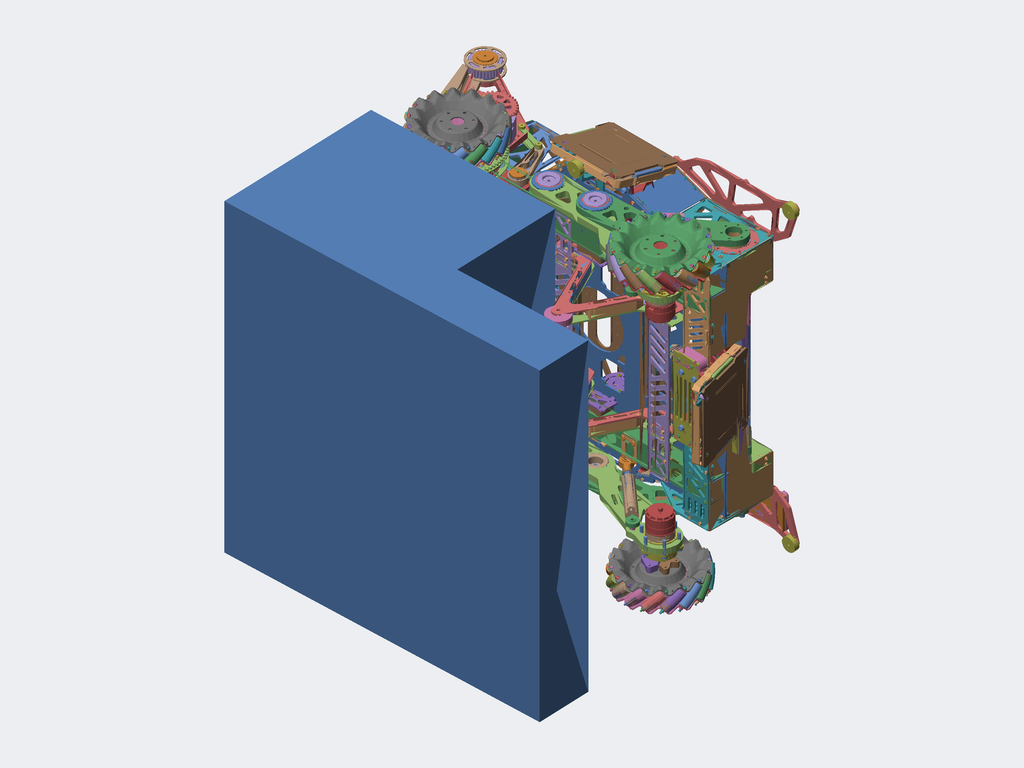Assembly | SolidWorks | 126 different items | 340 placed
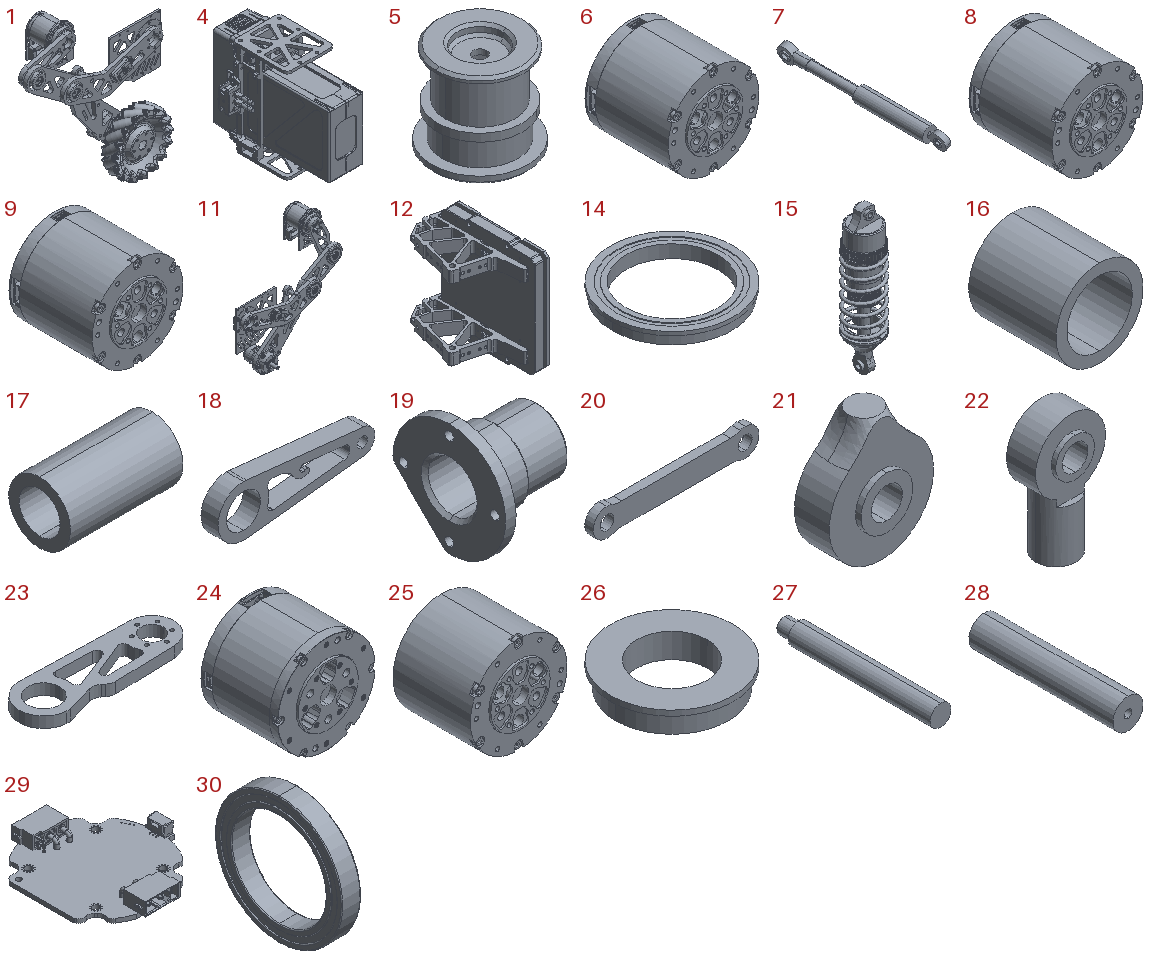Parts list (item | name | quantity | parent item | size | volume | features):
1 | (subassembly) | x1 | - | - | 882461 mm3 | -
2 | (subassembly) | x1 | - | - | - | features CompositeCurve 12, AEMSimFeature 1, CenterOfMass 1
3 | (subassembly) | x1 | in 2 | - | - | -
4 | (subassembly) | x1 | in 2 | - | 356333 mm3 | -
5 | (subassembly) | x4 | in 1, 11 | 37.15 x 37.15 x 35 mm | 13478 mm3 | -
6 | (subassembly) | x2 | in 9 | 57 x 53.3 x 57 mm | 118253 mm3 | -
7 | (subassembly) | x2 | in 1, 11 | - | 32855 mm3 | features CompositeCurve 1
8 | (subassembly) | x2 | in 1, 11 | 57 x 53.3 x 57 mm | 118253 mm3 | -
9 | (subassembly) | x2 | in 8 | 57 x 53.3 x 57 mm | 118253 mm3 | -
10 | (subassembly) | x1 | - | - | - | features CompositeCurve 8
11 | (subassembly) | x1 | - | - | 699438 mm3 | features CompositeCurve 1
12 | (subassembly) | x4 | in 2 | 74.786 x 139.379 x 141 mm | 156127 mm3 | -
13 | (subassembly) | x1 | - | - | - | features CompositeCurve 3
14 | - | x4 | in 10, 13 | 67 x 67 x 7 mm | 9465 mm3 | features ICE 1, Revolution 1
15 | - | x4 | in 10, 13 | 22.605 x 22.6 x 94.05 mm | 15306 mm3 | features BaseBody 4
16 | - | x1 | in 11 | 8 x 8 x 8 mm | 175.929 mm3 | features Extrusion 1
17 | - | x2 | in 1, 11 | 22 x 12 x 12 mm | 1382 mm3 | features Revolution 1
18 | - | x2 | in 10, 13 | 92.5 x 10 x 30 mm | 11719 mm3 | features Fillet 3, ICE 2, Extrusion 1
19 | - | x2 | in 10, 13 | 25 x 31.997 x 31.997 mm | 4923 mm3 | features Chamfer 2, HoleWzd 2, ICE 2, 3DProfileFeature 1, Fillet 1, Revolution 1
20 | - | x4 | in 10, 13 | 60 x 3 x 10 mm | 1346 mm3 | features Extrusion 1, Fillet 1
21 | - | x2 | in 7 | - | 2238 mm3 | features ICE 3, Extrusion 1, Fillet 1
22 | - | x2 | in 7 | 21.7 x 12.5 x 38.85 mm | 4732 mm3 | features ICE 4, Extrusion 1, HoleWzd 1
23 | - | x2 | in 1, 11 | 141.575 x 45.127 x 10 mm | 33796 mm3 | features ICE 3, Fillet 2, Extrusion 1
24 | - | x2 | in 10, 13 | 57 x 46 x 57 mm | 102676 mm3 | features BaseBody 10
25 | - | x2 | in 6 | 57 x 46.8 x 57 mm | 109300 mm3 | features BaseBody 1
26 | - | x4 | in 10, 13 | 35 x 35 x 7 mm | 3667 mm3 | features Extrusion 1, ICE 1
27 | - | x2 | in 7 | 11 x 83 x 11 mm | 7524 mm3 | features Extrusion 1, ICE 1, StudWizard 1
28 | - | x2 | in 7 | 19 x 91 x 19 mm | 18359 mm3 | features Extrusion 1, HoleWzd 1, ICE 1
29 | - | x2 | in 6 | - | - | features RefSurface 1
30 | - | x2 | in 1, 11 | 7 x 47 x 47 mm | 4099 mm3 | features Revolution 5, CirPattern 2, RefAxis 1, RevCut 1
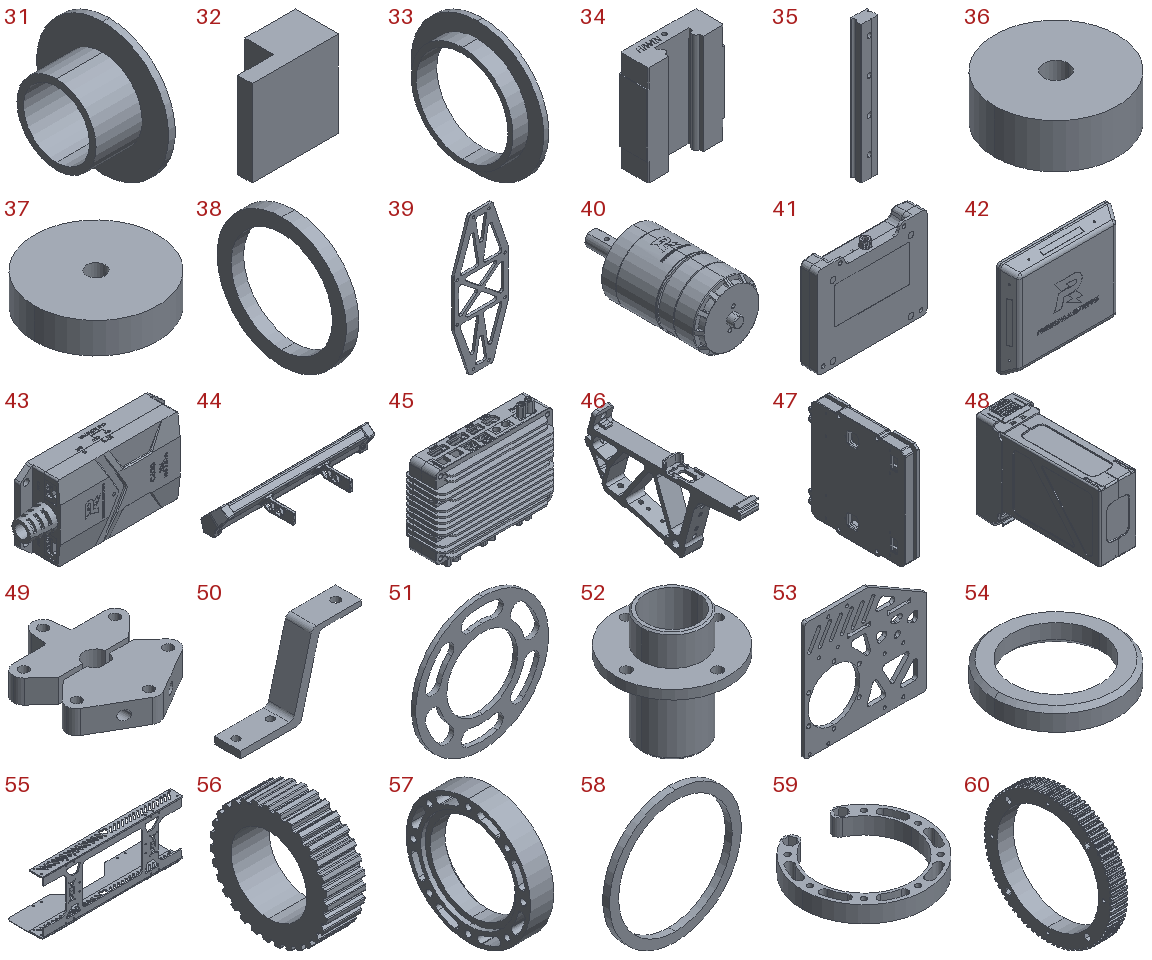31 | - | x8 | in 10, 13 | 4 x 10 x 10 mm | 59.69 mm3 | features Revolution 1
32 | - | x1 | - | 600 x 300 x 600 mm | 78000000 mm3 | features Extrusion 1
33 | - | x4 | in 10, 13 | 4 x 26 x 26 mm | 455.531 mm3 | features Revolution 1
34 | - | x8 | in 10, 13 | 27 x 10 x 34.7 mm | 7013 mm3 | features BaseBody 1
35 | - | x4 | in 10, 13 | 12 x 8 x 100 mm | 8420 mm3 | features ICE 3, BaseBody 1
36 | - | x4 | in 2 | 25 x 25 x 9 mm | 4241 mm3 | features Revolution 1
37 | - | x2 | in 2 | 40 x 40 x 10 mm | 12284 mm3 | features Revolution 1
38 | - | x2 | in 1, 11 | 5 x 51 x 51 mm | 3931 mm3 | features Revolution 1
39 | - | x1 | in 2 | 70 x 3 x 180 mm | 15170 mm3 | features ICE 2, Extrusion 1, Fillet 1
40 | - | x4 | in 1, 10, 11, 13 | 42 x 98.4 x 44.727 mm | 85611 mm3 | features BaseBody 17
41 | - | x1 | in 2 | 76 x 15.355 x 63 mm | 45153 mm3 | features BaseBody 13, DeleteBody 1, Revolution 1
42 | - | x1 | in 2 | 121.675 x 17.8 x 105.675 mm | 74088 mm3 | features BaseBody 6
43 | - | x4 | in 1, 2, 11 | 53.7 x 11.5 x 26.125 mm | 11767 mm3 | features BaseBody 25, DeleteBody 2, RefSurface 1
44 | - | x1 | in 2 | 285 x 84.728 x 49.99 mm | 138655 mm3 | features BaseBody 32, SewRefSurface 2, Thicken 2, DeleteBody 1, ICE 1
45 | - | x1 | in 2 | - | - | features BaseBody 45, RefSurface 2, DeleteBody 1
46 | - | x8 | in 12 | 15 x 130.973 x 68.389 mm | 25082 mm3 | features BaseBody 1
47 | - | x4 | in 12 | 19 x 129.965 x 141 mm | 105960 mm3 | features BaseBody 16, Blend 1, Shell 1
48 | - | x1 | in 4 | 44.3 x 134.8 x 101.5 mm | 316528 mm3 | features BaseBody 10
49 | - | x4 | in 1, 10, 11, 13 | 47.971 x 54.2 x 10 mm | 13527 mm3 | features BaseBody 2
50 | - | x2 | in 2 | 70.55 x 15 x 45 mm | 6219 mm3 | features Extrusion 1, Fillet 1, ICE 1
51 | - | x4 | in 10, 13 | 60 x 2 x 60 mm | 2573 mm3 | features Extrusion 1, ICE 1
52 | - | x2 | in 10, 13 | 37 x 37 x 36.5 mm | 6267 mm3 | features ICE 4, Chamfer 2, HoleWzd 2, 3DProfileFeature 1, Extrusion 1
53 | - | x2 | in 1, 11 | 130 x 4 x 126 mm | 41493 mm3 | features ICE 5, Fillet 2, Extrusion 1
54 | - | x8 | in 5 | 38 x 38 x 6.3 mm | 3255 mm3 | features Chamfer 2, Extrusion 1
55 | - | x1 | in 2 | 363 x 91.15 x 140 mm | 130923 mm3 | features ICE 5, Fillet 2, Extrusion 1, MirrorSolid 1
56 | - | x2 | in 10, 13 | 16 x 49.566 x 49.615 mm | 16375 mm3 | features CirPattern 1, Cut 1, ICE 1, RefAxis 1, Revolution 1
57 | - | x1 | in 10 | 16 x 85 x 85 mm | 32635 mm3 | features ICE 1, Revolution 1
58 | - | x2 | in 10, 13 | 58 x 3 x 58 mm | 2036 mm3 | features Extrusion 1
59 | - | x1 | in 10 | 74 x 70.267 x 10 mm | 10018 mm3 | features ICE 2, Extrusion 1, Fillet 1
60 | - | x2 | in 10, 13 | 16 x 125.578 x 125.622 mm | 66600 mm3 | features ICE 3, Cut 2, Chamfer 1, CirPattern 1, RefAxis 1, Revolution 1
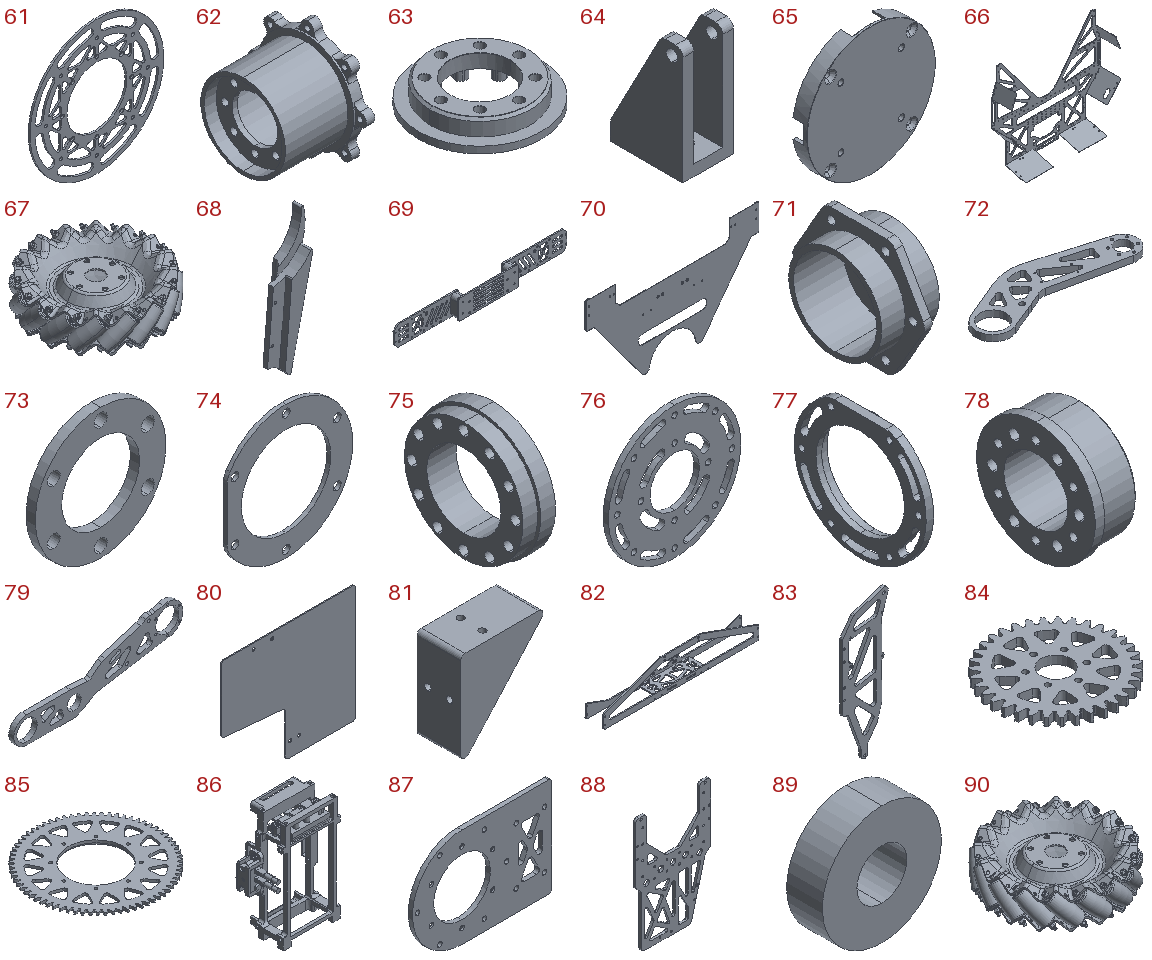61 | - | x4 | in 10, 13 | 145 x 2 x 145 mm | 15235 mm3 | features CirPattern 1, Extrusion 1, Fillet 1, ICE 1
62 | - | x2 | in 10, 13 | 43 x 70 x 70 mm | 21080 mm3 | features ICE 4, HoleWzd 1, Revolution 1
63 | - | x1 | in 10 | 55 x 55 x 10.2 mm | 10014 mm3 | features ICE 3, Chamfer 1, Fillet 1, Revolution 1
64 | - | x4 | in 10, 13 | 14 x 20 x 32 mm | 3086 mm3 | features ICE 4, Extrusion 1, Fillet 1
65 | - | x2 | in 6 | 57 x 6.5 x 57 mm | 5262 mm3 | features BaseBody 1
66 | - | x1 | in 2 | 486 x 96.259 x 428.466 mm | 244289 mm3 | features ICE 8, Fillet 4, Extrusion 1, MirrorSolid 1
67 | - | x2 | in 11, 13 | 152.394 x 152.394 x 45.547 mm | 219061 mm3 | features BaseBody 146
68 | - | x2 | in 10, 13 | 70.208 x 32 x 213.495 mm | 127310 mm3 | features ICE 3, Fillet 2, DelFace 1, Extrusion 1, MirrorSolid 1
69 | - | x1 | in 2 | 433.1 x 23 x 50 mm | 82463 mm3 | features ICE 8, Fillet 7, Chamfer 1, Extrusion 1
70 | - | x1 | in 2 | 441.1 x 3 x 236.71 mm | 53782 mm3 | features ICE 2, Extrusion 1, Fillet 1, MirrorSolid 1
71 | - | x2 | in 1, 11 | 29.45 x 67.158 x 59.5 mm | 18545 mm3 | features ICE 3, Fillet 1, Revolution 1
72 | - | x2 | in 1, 11 | 255.5 x 84.429 x 10 mm | 83626 mm3 | features ICE 7, Fillet 2, Extrusion 1
73 | - | x2 | in 1, 11 | 42 x 3 x 42 mm | 2434 mm3 | features Extrusion 1
74 | - | x2 | in 1, 11 | 66 x 2 x 70 mm | 3883 mm3 | features Extrusion 1
75 | - | x2 | in 1, 11 | 9.95 x 42 x 42 mm | 7242 mm3 | features HoleWzd 1, Revolution 1
76 | - | x2 | in 10, 13 | 75 x 3 x 75 mm | 8695 mm3 | features Extrusion 1, ICE 1
77 | - | x2 | in 1, 11 | 8 x 70 x 66 mm | 7364 mm3 | features ICE 2, Chamfer 1, Fillet 1, HoleWzd 1, Revolution 1
78 | - | x2 | in 1, 11 | 14 x 37 x 37 mm | 7882 mm3 | features ICE 2, Chamfer 1, HoleWzd 1, Revolution 1
79 | - | x2 | in 1, 11 | 347.966 x 10 x 110.45 mm | 118705 mm3 | features ICE 5, Fillet 2, Extrusion 1
80 | - | x2 | in 2 | 144.55 x 1 x 127 mm | 14747 mm3 | features Extrusion 1, Fillet 1
81 | - | x2 | in 2 | 37.777 x 20 x 41.764 mm | 17216 mm3 | features ICE 2, Extrusion 1, Fillet 1
82 | - | x1 | in 2 | 433.1 x 53 x 95 mm | 77453 mm3 | features Fillet 6, ICE 4, Extrusion 1
83 | - | x2 | in 2 | 81.5 x 5 x 248 mm | 38824 mm3 | features Fillet 3, ICE 3, Chamfer 1, Extrusion 1
84 | - | x2 | in 10, 13 | 73.978 x 73.911 x 5 mm | 13896 mm3 | features ICE 3, CirPattern 1, Extrusion 1, RefAxis 1
85 | - | x2 | in 10, 13 | 144 x 143.917 x 5 mm | 31123 mm3 | features ICE 4, CirPattern 1, Extrusion 1, HoleWzd 1, RefAxis 1
86 | - | x1 | in 4 | 69.4 x 39.5 x 103.5 mm | 27545 mm3 | features BaseBody 12
87 | - | x2 | in 1, 11 | 98.2 x 3 x 70 mm | 13699 mm3 | features ICE 2, 3DProfileFeature 1, Extrusion 1, Fillet 1, HoleWzd 1
88 | - | x2 | in 10, 13 | 133 x 4 x 208.15 mm | 51561 mm3 | features ICE 8, Fillet 4, Chamfer 1, Extrusion 1
89 | - | x2 | in 2 | 10 x 3 x 10 mm | 194.056 mm3 | features Extrusion 1
90 | - | x2 | in 1, 10 | 152.18 x 152.18 x 45.547 mm | 218308 mm3 | features BaseBody 114, ICE 1
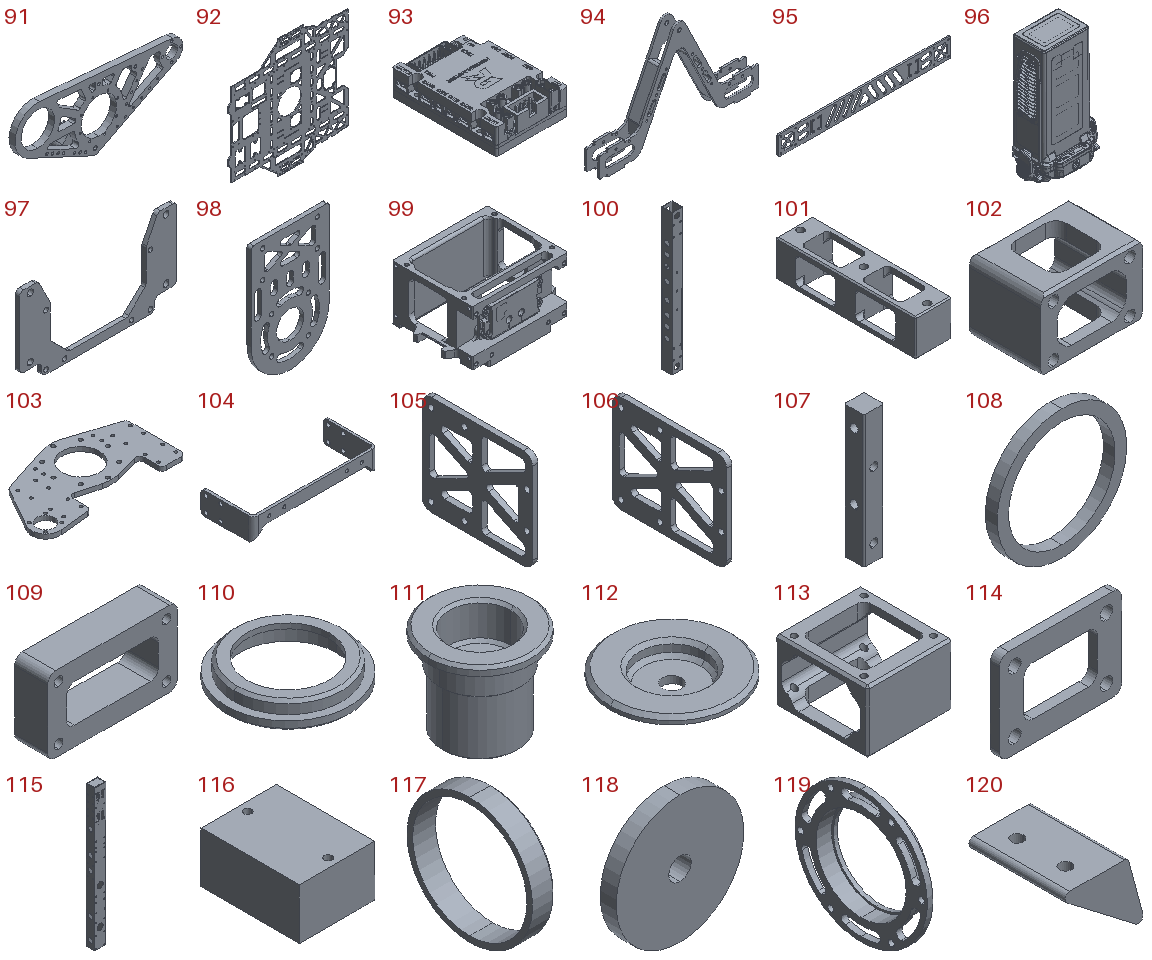91 | - | x2 | in 10, 13 | 276 x 41 x 121.736 mm | 133233 mm3 | features ICE 8, Fillet 5, Extrusion 1, MirrorSolid 1
92 | - | x1 | in 2 | 510.5 x 3 x 508 mm | 398593 mm3 | features ICE 16, Fillet 6, Chamfer 2, Extrusion 1
93 | - | x1 | in 2 | - | 22685 mm3 | features BaseBody 8
94 | - | x2 | in 2 | 239 x 22 x 147.217 mm | 68653 mm3 | features ICE 5, Extrusion 1, Fillet 1, MirrorSolid 1
95 | - | x2 | in 2 | 355 x 3 x 40 mm | 28604 mm3 | features ICE 3, Extrusion 1, Fillet 1
96 | - | x1 | in 3 | - | - | features RefSurface 17, Attribute 3
97 | - | x1 | in 2 | 110 x 3 x 59 mm | 7718 mm3 | features Chamfer 2, Extrusion 1, Fillet 1
98 | - | x2 | in 1, 11 | 57 x 3 x 91.7 mm | 10337 mm3 | features Extrusion 1, Fillet 1, ICE 1
99 | - | x1 | in 3 | - | - | features BaseBody 126, RefSurface 28, Attribute 3
100 | - | x2 | in 2 | 30 x 30 x 415 mm | 44267 mm3 | features ICE 3, Extrusion 1, Shell 1
101 | - | x2 | in 2 | 28 x 106 x 28 mm | 37370 mm3 | features ICE 2, Chamfer 1, Extrusion 1
102 | - | x4 | in 2 | 40 x 28 x 28 mm | 13306 mm3 | features ICE 3, Fillet 2, Chamfer 1, Extrusion 1
103 | - | x2 | in 10, 13 | 163.5 x 91 x 5 mm | 40085 mm3 | features ICE 10, Fillet 5, MirrorPattern 2, Extrusion 1
104 | - | x1 | in 2 | 100 x 41.788 x 18 mm | 4551 mm3 | features Fillet 1, FlatPattern 1, HoleWzd 1, SM3dBend 1, SMBaseFlange 1, SheetMetal 1
105 | - | x1 | in 4 | 3 x 61 x 55 mm | 5958 mm3 | features Fillet 2, ICE 2, Extrusion 1
106 | - | x1 | in 4 | 3 x 64.5 x 55 mm | 6303 mm3 | features Fillet 2, ICE 2, Extrusion 1
107 | - | x50 | in 2, 10 | 6 x 6 x 40 mm | 1314 mm3 | features HoleWzd 2, Extrusion 1, Fillet 1
108 | - | x4 | in 5 | 33 x 3 x 33 mm | 829.092 mm3 | features Extrusion 1
109 | - | x2 | in 1, 11 | 48 x 12.25 x 28 mm | 10214 mm3 | features Extrusion 1
110 | - | x8 | in 5 | 48 x 48 x 8.3 mm | 4148 mm3 | features Chamfer 2, ICE 2, Extrusion 1
111 | - | x4 | in 5 | 37.15 x 37.15 x 32.5 mm | 10461 mm3 | features Chamfer 5, ICE 4, 3DProfileFeature 1, Extrusion 1, HoleWzd 1
112 | - | x4 | in 5 | 34 x 34 x 6 mm | 2188 mm3 | features Chamfer 2, ICE 2, Extrusion 1
113 | - | x4 | in 2 | 37 x 40 x 27 mm | 11447 mm3 | features ICE 3, 3DProfileFeature 1, Chamfer 1, Extrusion 1, HoleWzd 1
114 | - | x4 | in 2 | 40 x 3 x 30 mm | 2282 mm3 | features Extrusion 1
115 | - | x2 | in 2 | 40 x 30 x 505 mm | 171270 mm3 | features ICE 9, Chamfer 1, Extrusion 1, Fillet 1
116 | - | x2 | in 2 | 44.5 x 58 x 30 mm | 76476 mm3 | features Extrusion 1
117 | - | x4 | in 10, 13 | 10 x 55 x 55 mm | 4038 mm3 | features Chamfer 1, Revolution 1
118 | - | x4 | in 10, 13 | 24 x 3 x 24 mm | 1316 mm3 | features Extrusion 1
119 | - | x2 | in 1, 11 | 10 x 69 x 69 mm | 6569 mm3 | features ICE 2, Revolution 1
120 | - | x2 | in 2 | 16.208 x 20 x 12.902 mm | 1998 mm3 | features Extrusion 1, Fillet 1, HoleWzd 1, MirrorPattern 1
121 | hex nuts, style 1-grades ab gb | x1 | - | - | - | -
122 | hexagon socket button head screws gb | x1 | - | - | - | -
123 | hexagon socket countersunk head screws gb | x1 | - | - | - | -
124 | hexagon socket head cap screws gb | x1 | - | - | - | -
125 | hexagon socket head shoulder screws gb | x1 | - | - | - | -
126 | Shoulder Bolt | x1 | - | - | - | -
Mates (type | each side: item.copy, entity, surface, feature), first 384 of 755 lines:
In the top assembly
Coincident | 115.1 face plane Boss-Extrude 1 | 88.1 face plane Boss-Extrude 1
Concentric | 115.1 face cylinder Cut-Extrude 2 | 88.1 face cylinder Cut-Extrude 3
Concentric | 115.1 face cylinder Cut-Extrude 2 | 15.1 face cylinder Shock Absorber-85mm Thickened Center Shaft-1-solid1
Coincident | 115.2 face plane Boss-Extrude 1 | 88.2 face plane Boss-Extrude 1
Concentric | 115.2 face cylinder Cut-Extrude 2 | 15.2 face cylinder Shock Absorber-85mm Thickened Center Shaft-1-solid1
Concentric | 115.2 face cylinder Cut-Extrude 2 | 15.3 face cylinder Shock Absorber-85mm Thickened Center Shaft-1-solid1
Coincident | 115.1 face plane Boss-Extrude 1 | 87.1 face plane Boss-Extrude 1
Concentric | 115.1 face cylinder Cut-Extrude 4 | 87.1 face cylinder Boss-Extrude 1 | 2 times
Concentric | 107.1 face cylinder M3 Tapped Hole 2 | 53.1 face cylinder Boss-Extrude 1
Coincident | 115.2 face plane Boss-Extrude 1 | 87.2 face plane Boss-Extrude 1
Concentric | 115.2 face cylinder Cut-Extrude 4 | 87.2 face cylinder Boss-Extrude 1 | 2 times
Concentric | 107.2 face cylinder M3 Tapped Hole 2 | 53.2 face cylinder Boss-Extrude 1 | 2 times
Concentric | 107.3 face cylinder M3 Tapped Hole 1 | 53.1 face cylinder Cut-Extrude 1 | 2 times
Concentric | 107.4 face cylinder M3 Tapped Hole 2 | 53.2 face cylinder Cut-Extrude 1
Concentric | 72.1 face cylinder Boss-Extrude 1 | 72.2 face cylinder Boss-Extrude 1
Concentric | 91.1 face cylinder Boss-Extrude 1 | 91.2 face cylinder Boss-Extrude 1
Coincident | 100.1 face plane Boss-Extrude 1 | assembly face
Coincident | 2.1 plane | 32.1 plane
Tangent | 37.1 face cylinder Revolve 1 | 32.1 face plane Boss-Extrude 1
Tangent | 90.1 select_type:24 | 32.1 face plane Boss-Extrude 1
Parallel | 92.1 select_type:24 | 32.1 face plane Boss-Extrude 1
Concentric | 115.2 face cylinder Cut-Extrude 3 | assembly face
Coincident | 115.2 face plane Boss-Extrude 1 | assembly face
Coincident | 53.2 face plane Boss-Extrude 1 | assembly face | 2 times
Concentric | 53.2 face cylinder Boss-Extrude 1 | assembly face
Coincident | 88.2 face plane Boss-Extrude 1 | assembly face
Concentric | 100.1 face cylinder Cut-Extrude 1 | assembly face | 2 times
In subassembly 2
Coincident | 92.2 face plane Boss-Extrude 1 | 115.3 face plane Boss-Extrude 1
Coincident | 92.2 face plane Boss-Extrude 1 | 115.4 face plane Boss-Extrude 1
Coincident | 115.3 face plane Boss-Extrude 1 | 2.2 face | 3 times
Concentric | 115.3 face cylinder Cut-Extrude 2 | 2.2 face | 4 times
Concentric | 2.2 face | 2.2 face | 10 times
Coincident | 115.4 face plane Boss-Extrude 1 | 2.2 face | 2 times
Concentric | 115.4 face cylinder Cut-Extrude 2 | 2.2 face | 3 times
Concentric | 2.2 face | 107.5 face cylinder M3 Tapped Hole 2 | 2 times
Coincident | 2.2 face | 107.5 face plane Boss-Extrude 1
Coincident | 2.2 face | 2.2 face | 9 times
Concentric | 92.2 face cylinder Cut-Extrude 1 | 46.1 face cylinder Import 1
Concentric | 92.2 face cylinder Cut-Extrude 1 | 46.2 face cylinder Import 1
Coincident | 2.2 edge | 2.2 edge
Concentric | 92.2 face cylinder Cut-Extrude 2 | 115.3 face cylinder Cut-Extrude 3 | 2 times
Coincident | 92.2 face plane Boss-Extrude 1 | 46.1 face plane Import 1
Concentric | 2.2 face | 55.1 face cylinder Mirror 1 | 2 times
Concentric | 92.2 face cylinder Cut-Extrude 2 | 115.4 face cylinder Cut-Extrude 3 | 2 times
Concentric | 55.1 face cylinder Boss-Extrude 2 | 2.2 face | 3 times
Concentric | 55.1 face cylinder Boss-Extrude 2 | 107.6 face cylinder M3 Tapped Hole 1 | 2 times
Concentric | 2.2 face | 107.6 face cylinder M3 Tapped Hole 2
Coincident | 2.2 face | 55.1 face plane Mirror 1
Coincident | 92.2 face plane Boss-Extrude 1 | 2.2 face | 6 times
Coincident | 46.2 face plane Import 1 | 46.3 face plane Import 1
Tangent | 2.2 select_type:0 | 2.2 face
Concentric | 115.3 face cylinder Cut-Extrude 4 | 2.2 face | 2 times
Coincident | 92.2 face plane Boss-Extrude 1 | 46.4 face plane Import 1
Concentric | 92.2 face cylinder Boss-Extrude 2 | 46.4 face cylinder Import 1
Concentric | 92.2 face cylinder Boss-Extrude 2 | 46.5 face cylinder Import 1
Coincident | 92.2 select_type:24 | 2.2 face | 2 times
Coincident | 2.2 plane | 2.2 plane
Concentric | 46.3 face cylinder Import 1 | 2.2 face | 2 times
Coincident | 92.2 face plane Boss-Extrude 1 | 100.2 face plane Boss-Extrude 1
Coincident | 92.2 face plane Boss-Extrude 1 | 100.3 face plane Boss-Extrude 1
Coincident | 92.2 face plane Boss-Extrude 2 | 100.3 face plane Boss-Extrude 1
Parallel | 46.6 face plane Import 1 | 44.1 face plane Import 22 | 2 times
Concentric | 46.3 face cylinder Import 1 | 69.1 face cylinder Boss-Extrude 3
Concentric | 46.6 face cylinder Import 1 | 69.1 face cylinder Boss-Extrude 3
Coincident | 46.6 face plane Import 1 | 69.1 face plane Boss-Extrude 3
Coincident | 115.3 face plane Boss-Extrude 1 | 69.1 face plane Boss-Extrude 1
Coincident | 55.1 face plane Boss-Extrude 2 | 2.2 face
Coincident | 55.1 face plane Boss-Extrude 2 | 107.6 face plane Boss-Extrude 1
Concentric | 107.5 face cylinder M3 Tapped Hole 1 | 55.1 face cylinder Mirror 1 | 2 times
Coincident | 107.5 face plane Boss-Extrude 1 | 55.1 face plane Mirror 1
Concentric | 69.1 face cylinder Cut-Extrude 1 | 107.7 edge
Concentric | 2.2 face | 107.7 face cylinder M3 Tapped Hole 2
Concentric | 92.2 face cylinder Cut-Extrude 4 | 107.8 face cylinder M3 Tapped Hole 1 | 2 times
Concentric | 2.2 face | 107.8 face cylinder M3 Tapped Hole 2
Concentric | 46.6 face cylinder Import 1 | 82.1 face cylinder Boss-Extrude 1 | 2 times
Coincident | 46.6 face plane Import 1 | 82.1 face plane Boss-Extrude 1
Coincident | 82.1 face plane Boss-Extrude 1 | 2.2 face
Parallel | 46.1 face plane Import 1 | 86.1 face plane DJI Battery Holder 2017-1-solid1
Coincident | 82.1 face plane Boss-Extrude 1 | 107.9 face plane Boss-Extrude 1
Concentric | 82.1 face cylinder Cut-Extrude 1 | 107.9 edge
Concentric | 82.1 face cylinder Boss-Extrude 2 | 107.9 face cylinder M3 Tapped Hole 2
Coincident | 82.1 face plane Boss-Extrude 3 | 104.1 face plane Base-Flange 1
Coincident | 44.1 face plane Import 22 | 82.1 face plane Boss-Extrude 2
Concentric | 82.1 face cylinder Boss-Extrude 3 | 104.1 face cylinder M3 Tapped Hole 2 | 2 times
Coincident | 44.1 face plane Import 22 | 104.1 face plane Sketched Bend 2
Concentric | 44.1 face cylinder Cut-Extrude 1 | 104.1 face cylinder Base-Flange 1 | 2 times
Coincident | 82.1 face plane Boss-Extrude 1 | 107.10 face plane Boss-Extrude 1
Concentric | 82.1 face cylinder Boss-Extrude 2 | 107.10 face cylinder M3 Tapped Hole 1
Concentric | 82.1 face cylinder Cut-Extrude 1 | 107.10 face cylinder M3 Tapped Hole 2
Coincident | 82.1 face plane Boss-Extrude 2 | 107.11 face plane Boss-Extrude 1
Concentric | 82.1 face cylinder Boss-Extrude 3 | 107.11 face cylinder M3 Tapped Hole 2
Concentric | 82.1 face cylinder Boss-Extrude 2 | 107.11 face cylinder M3 Tapped Hole 1
Concentric | 82.1 face cylinder Boss-Extrude 2 | 107.12 face cylinder M3 Tapped Hole 2
Concentric | 82.1 face cylinder Boss-Extrude 3 | 107.12 face cylinder M3 Tapped Hole 1
Coincident | 92.2 face plane Boss-Extrude 1 | 107.8 face plane Boss-Extrude 1
Concentric | 82.1 face cylinder Boss-Extrude 3 | 107.13 face cylinder M3 Tapped Hole 2 | 2 times
Coincident | 82.1 face plane Boss-Extrude 3 | 107.13 face plane Boss-Extrude 1
Coincident | 82.1 face plane Boss-Extrude 1 | 107.14 face plane Boss-Extrude 1
Concentric | 82.1 face cylinder Cut-Extrude 1 | 107.14 face cylinder M3 Tapped Hole 2 | 2 times
Concentric | 46.4 face cylinder Import 1 | 66.1 face cylinder Boss-Extrude 1
Concentric | 46.2 face cylinder Import 1 | 66.1 face cylinder Boss-Extrude 1
Coincident | 46.5 face plane Import 1 | 66.1 face plane Boss-Extrude 1
Coincident | 2.2 face | 107.15 face plane Boss-Extrude 1
Concentric | 46.1 face cylinder Import 1 | 97.1 face cylinder Boss-Extrude 1 | 2 times
Coincident | 46.2 face plane Import 1 | 97.1 face plane Boss-Extrude 1
Coincident | 92.2 face plane Boss-Extrude 1 | 46.7 face plane Import 1
Concentric | 92.2 face cylinder Boss-Extrude 2 | 46.7 face cylinder Import 1 | 2 times
Coincident | 92.2 select_type:25 | 2.2 axis | 2 times
Coincident | 100.3 face plane Boss-Extrude 1 | 2.2 face | 4 times
Concentric | 100.3 face cylinder Cut-Extrude 1 | 2.2 face | 3 times
Concentric | 100.3 edge | 2.2 face
Concentric | 100.2 face cylinder Cut-Extrude 1 | 2.2 face | 2 times
Concentric | 92.2 face cylinder Cut-Extrude 6 | 100.2 face cylinder Cut-Extrude 1 | 2 times
Concentric | 92.2 face cylinder Cut-Extrude 6 | 100.3 face cylinder Cut-Extrude 1
Coincident | 66.1 face plane Boss-Extrude 3 | 107.16 face plane Boss-Extrude 1
Concentric | 66.1 face cylinder Boss-Extrude 3 | 107.16 face cylinder M3 Tapped Hole 2 | 2 times
Concentric | 2.2 face | 107.15 face cylinder M3 Tapped Hole 1 | 2 times
Concentric | 107.15 face cylinder M3 Tapped Hole 2 | 70.1 face cylinder Boss-Extrude 1 | 2 times
Coincident | 107.15 face plane Boss-Extrude 1 | 70.1 face plane Boss-Extrude 1
Coincident | 69.1 face plane Boss-Extrude 1 | 80.1 face plane Boss-Extrude 1
Coincident | 66.1 face plane Boss-Extrude 5 | 120.1 face plane Boss-Extrude 1
Concentric | 66.1 face cylinder Cut-Extrude 2 | 120.1 face cylinder Mirror 1 | 2 times
Coincident | 99.1 face plane battery_rack.stp-1/_V06-202409130001_ASM_12_ASM.stp-1/DCJ-V13-20241024_13.stp-1-solid1 | 97.1 face plane Boss-Extrude 1
Concentric | 99.1 face cylinder battery_rack.stp-1/_V06-202409130001_ASM_12_ASM.stp-1/DCJ-V13-20241024_13.stp-1-solid1 | 97.1 face cylinder Boss-Extrude 1 | 2 times
Coincident | 80.1 face plane Boss-Extrude 1 | 81.1 face plane Boss-Extrude 1
Coincident | 70.1 face plane Boss-Extrude 1 | 81.1 face plane Boss-Extrude 1 | 2 times
Concentric | 80.1 face cylinder Boss-Extrude 1 | 81.1 face cylinder Cut-Extrude 2 | 2 times
Concentric | 69.1 face cylinder Boss-Extrude 1 | 107.17 face cylinder M3 Tapped Hole 1
Concentric | 80.1 face cylinder Boss-Extrude 1 | 107.17 face cylinder M3 Tapped Hole 2
Concentric | 69.1 face cylinder Boss-Extrude 1 | 107.18 face cylinder M3 Tapped Hole 2 | 2 times
Coincident | 69.1 face plane Boss-Extrude 1 | 107.18 face plane Boss-Extrude 1
Concentric | 80.2 face cylinder Boss-Extrude 1 | 107.18 face cylinder M3 Tapped Hole 1 | 2 times
Coincident | 80.2 face plane Boss-Extrude 1 | 107.18 face plane Boss-Extrude 1
Coincident | 80.2 face plane Boss-Extrude 1 | 81.2 face plane Boss-Extrude 1
Concentric | 80.2 face cylinder Boss-Extrude 1 | 81.2 face cylinder Cut-Extrude 2 | 2 times
Coincident | 66.1 face plane Boss-Extrude 1 | 83.1 face plane Boss-Extrude 1
Concentric | 70.1 face cylinder Boss-Extrude 1 | 83.1 face cylinder Boss-Extrude 1
Concentric | 46.5 face cylinder Import 1 | 83.1 face cylinder Boss-Extrude 1
Coincident | 83.1 face plane Boss-Extrude 1 | 41.1 face plane Import 5
Concentric | 83.1 face cylinder Boss-Extrude 2 | 41.1 face cylinder Import 5
Concentric | 83.1 face cylinder Cut-Extrude 3 | 41.1 face cylinder Import 5
Concentric | 46.8 face cylinder Import 1 | 83.2 face cylinder Boss-Extrude 1
Concentric | 70.1 face cylinder Boss-Extrude 1 | 83.2 face cylinder Boss-Extrude 1
Coincident | 66.1 face plane Boss-Extrude 1 | 83.2 face plane Boss-Extrude 1
Coincident | 83.1 face plane Boss-Extrude 1 | 36.1 face plane Revolve 1
Concentric | 83.1 face cylinder Boss-Extrude 1 | 36.1 edge
Coincident | 92.2 face plane Boss-Extrude 1 | 50.1 face plane Boss-Extrude 1
Concentric | 92.2 face cylinder Boss-Extrude 2 | 50.1 face cylinder Cut-Extrude 1 | 2 times
Concentric | 50.1 face cylinder Cut-Extrude 1 | 36.2 face cylinder Revolve 1
Coincident | 92.2 face plane Boss-Extrude 1 | 50.2 face plane Boss-Extrude 1
Concentric | 92.2 face cylinder Boss-Extrude 2 | 50.2 face cylinder Cut-Extrude 1 | 2 times
Coincident | 50.2 face plane Boss-Extrude 1 | 36.3 face plane Revolve 1
Concentric | 50.2 face cylinder Cut-Extrude 1 | 36.3 face cylinder Revolve 1
Coincident | 92.2 face plane Boss-Extrude 1 | 94.1 face plane Boss-Extrude 1
Coincident | 92.2 face plane Support Guide Wheel Mount | 94.1 face plane Boss-Extrude 1 | 2 times
Tangent | 2.2 face | 94.1 select_type:24
Concentric | 115.3 face cylinder Cut-Extrude 3 | 95.1 face cylinder Boss-Extrude 1 | 2 times
Coincident | 115.3 face plane Boss-Extrude 1 | 95.2 face plane Boss-Extrude 1
Concentric | 115.3 face cylinder Cut-Extrude 3 | 95.2 face cylinder Boss-Extrude 1 | 2 times
Concentric | 94.1 face cylinder Boss-Extrude 1 | 2.2 face
Concentric | 94.2 face cylinder Boss-Extrude 1 | 2.2 face
Coincident | 95.1 face plane Boss-Extrude 1 | 2.2 face | 4 times
Coincident | 95.1 face plane Boss-Extrude 1 | 94.2 face plane Boss-Extrude 1 | 2 times
Concentric | 42.1 face cylinder Import 2 | 39.1 face cylinder Cut-Extrude 1 | 2 times
Coincident | 42.1 face plane Import 2 | 39.1 face plane Boss-Extrude 1
Concentric | 55.1 face cylinder Cut-Extrude 1 | 39.1 face cylinder Cut-Extrude 1 | 2 times
Coincident | 55.1 face plane Boss-Extrude 1 | 39.1 face plane Boss-Extrude 1
Concentric | 83.2 face cylinder Boss-Extrude 1 | 36.4 face cylinder Revolve 1
Coincident | 83.2 face plane Boss-Extrude 1 | 36.4 face plane Revolve 1
Width | 94.1 face plane Boss-Extrude 1 | 2.2 face | 37.2 face plane Revolve 1 | 37.2 face plane Revolve 1
Concentric | 2.2 face | 37.2 face cylinder Revolve 1
Concentric | 94.2 face cylinder Boss-Extrude 1 | 37.3 face cylinder Revolve 1
Width | 2.2 face | 94.2 face plane Boss-Extrude 1 | 37.3 face plane Revolve 1 | 37.3 face plane Revolve 1
Coincident | 50.1 face plane Boss-Extrude 1 | 36.2 face plane Revolve 1
Concentric | 95.1 face cylinder Cut-Extrude 2 | 107.19 face cylinder M3 Tapped Hole 1
Concentric | 94.1 face cylinder Cut-Extrude 3 | 107.19 face cylinder M3 Tapped Hole 2
Coincident | 94.1 face plane Mirror 1 | 95.1 face plane Boss-Extrude 1
Concentric | 94.1 face cylinder Boss-Extrude 1 | 37.2 face cylinder Revolve 1
Coincident | 95.1 face plane Boss-Extrude 1 | 94.2 face plane Mirror 1
Concentric | 100.2 face cylinder Cut-Extrude 1 | 102.1 face cylinder Cut-Extrude 1 | 2 times
Coincident | 100.2 face plane Shell 1 | 102.1 face plane Boss-Extrude 1
Coincident | 100.3 face plane Shell 1 | 102.2 face plane Boss-Extrude 1
Concentric | 100.3 face cylinder Cut-Extrude 1 | 102.2 face cylinder Cut-Extrude 1 | 2 times
Coincident | 115.3 face plane Boss-Extrude 1 | 113.1 face plane Boss-Extrude 1
Concentric | 115.3 face cylinder Cut-Extrude 3 | 113.1 face cylinder Cut-Extrude 3 | 2 times
Concentric | 100.2 face cylinder Cut-Extrude 1 | 101.1 face cylinder Cut-Extrude 1 | 2 times
Coincident | 100.2 face plane Shell 1 | 101.1 face plane Boss-Extrude 1
Concentric | 115.3 face cylinder Cut-Extrude 5 | 114.1 face cylinder Boss-Extrude 1 | 2 times
Coincident | 115.3 face plane Boss-Extrude 1 | 114.1 face plane Boss-Extrude 1
Concentric | 92.2 face cylinder Conduit Mount | 45.1 face cylinder Import 24 | 2 times
Coincident | 92.2 face plane Boss-Extrude 1 | 45.1 face plane Import 24
Concentric | 69.1 face cylinder Cut-Extrude 1 | 107.7 face cylinder M3 Tapped Hole 1
Coincident | 82.1 face plane Boss-Extrude 3 | 70.1 face plane Boss-Extrude 1
Concentric | 82.1 face cylinder Cut-Extrude 1 | 107.20 face cylinder M3 Tapped Hole 2 | 2 times
Coincident | 82.1 face plane Boss-Extrude 1 | 107.20 face plane Boss-Extrude 1
Coincident | 92.2 face plane Boss-Extrude 1 | 107.21 face plane Boss-Extrude 1
Concentric | 92.2 face cylinder Cut-Extrude 4 | 107.21 face cylinder M3 Tapped Hole 1 | 2 times
Coincident | 69.1 face plane Boss-Extrude 1 | 107.22 face plane Boss-Extrude 1
Concentric | 69.1 face cylinder Cut-Extrude 1 | 107.22 face cylinder M3 Tapped Hole 2 | 2 times
Concentric | 115.3 face cylinder Cut-Extrude 3 | 69.1 face cylinder Boss-Extrude 1
Concentric | 115.4 face cylinder Cut-Extrude 3 | 69.1 face cylinder Boss-Extrude 1
Coincident | 69.1 face plane Boss-Extrude 1 | 107.7 face plane Boss-Extrude 1
Coincident | 92.2 face plane Boss-Extrude 1 | 107.23 face plane Boss-Extrude 1
Concentric | 92.2 face cylinder Battery Mount | 107.23 face cylinder M3 Tapped Hole 2 | 2 times
Concentric | 105.1 face cylinder Cut-Extrude 1 | 107.23 face cylinder M3 Tapped Hole 1 | 2 times
Coincident | 105.1 face plane Boss-Extrude 1 | 107.23 face plane Boss-Extrude 1
Concentric | 92.2 face cylinder Electronics Mount | 2.2 face | 2 times
Coincident | 92.2 face plane Boss-Extrude 1 | 93.1 face plane 3_0-1-solid1
Concentric | 92.2 face cylinder Electronics Mount | 93.1 face cylinder 4_0-1-solid1
Concentric | 92.2 face cylinder Electronics Mount | 93.1 face cylinder 4_0-4-solid1
Concentric | 92.2 face cylinder Electronics Mount | 116.1 face cylinder Boss-Extrude 1 | 2 times
Concentric | 92.2 face cylinder Electronics Mount | 116.2 face cylinder Boss-Extrude 1 | 2 times
Coincident | 92.2 face plane Boss-Extrude 1 | 116.1 face plane Boss-Extrude 1
Concentric | 55.1 face cylinder Cut-Extrude 1 | 43.1 face cylinder C620 Brushless Motor ESC.STEP-1/7.STEP-1-solid1 | 2 times
Coincident | 55.1 face plane Boss-Extrude 1 | 43.1 face plane C620 Brushless Motor ESC.STEP-1/7.STEP-1-solid1
Coincident | 55.1 face plane Boss-Extrude 1 | 43.2 face plane C620 Brushless Motor ESC.STEP-1/7.STEP-1-solid1
Concentric | 55.1 face cylinder Cut-Extrude 1 | 43.2 face cylinder C620 Brushless Motor ESC.STEP-1/7.STEP-1-solid1 | 2 times
Concentric | 115.3 face cylinder Cut-Extrude 5 | 114.2 face cylinder Boss-Extrude 1 | 2 times
Coincident | 115.3 face plane Boss-Extrude 1 | 114.2 face plane Boss-Extrude 1
Concentric | 115.4 face cylinder Cut-Extrude 5 | 114.3 face cylinder Boss-Extrude 1 | 2 times
Coincident | 115.4 face plane Boss-Extrude 1 | 114.3 face plane Boss-Extrude 1
Concentric | 115.4 face cylinder Cut-Extrude 5 | 114.4 face cylinder Boss-Extrude 1 | 2 times
Coincident | 115.4 face plane Boss-Extrude 1 | 114.4 face plane Boss-Extrude 1
Coincident | 115.3 face plane Boss-Extrude 1 | 113.2 face plane Boss-Extrude 1
Concentric | 95.1 face cylinder Boss-Extrude 1 | 113.2 face cylinder Cut-Extrude 3 | 2 times
Coincident | 66.1 face plane Boss-Extrude 1 | 120.2 face plane Boss-Extrude 1
Concentric | 66.1 face cylinder Boss-Extrude 1 | 120.2 face cylinder M3 Tapped Hole 1 | 2 times
Coincident | 92.2 face plane Boss-Extrude 1 | 116.2 face plane Boss-Extrude 1
Concentric | 92.2 face cylinder Boss-Extrude 4 | 107.24 face cylinder M3 Tapped Hole 2 | 2 times
Concentric | 55.1 face cylinder Boss-Extrude 3 | 107.24 face cylinder M3 Tapped Hole 1 | 2 times
Concentric | 92.2 face cylinder Boss-Extrude 4 | 2.2 face | 2 times
Concentric | 55.1 face cylinder Boss-Extrude 3 | 2.2 face
Concentric | 92.2 face cylinder Boss-Extrude 4 | 107.25 face cylinder M3 Tapped Hole 1 | 2 times
Concentric | 55.1 face cylinder Boss-Extrude 3 | 107.25 face cylinder M3 Tapped Hole 2 | 2 times
Coincident | 92.2 face plane Boss-Extrude 1 | 107.25 face plane Boss-Extrude 1
Coincident | 92.2 face plane Boss-Extrude 1 | 107.24 face plane Boss-Extrude 1
Concentric | 66.1 face cylinder Boss-Extrude 2 | 107.26 face cylinder M3 Tapped Hole 2 | 2 times
Coincident | 66.1 face plane Boss-Extrude 2 | 107.26 face plane Boss-Extrude 1
Concentric | 66.1 face cylinder Boss-Extrude 2 | 107.27 face cylinder M3 Tapped Hole 2 | 2 times
Coincident | 66.1 face plane Boss-Extrude 2 | 107.27 face plane Boss-Extrude 1
Concentric | 66.1 face cylinder Boss-Extrude 3 | 107.28 face cylinder M3 Tapped Hole 2 | 2 times
Coincident | 66.1 face plane Boss-Extrude 3 | 107.28 face plane Boss-Extrude 1
Concentric | 55.1 face cylinder Boss-Extrude 2 | 107.29 face cylinder M3 Tapped Hole 2 | 2 times
Coincident | 55.1 face plane Boss-Extrude 2 | 107.29 face plane Boss-Extrude 1
Concentric | 55.1 face cylinder Boss-Extrude 2 | 107.30 face cylinder M3 Tapped Hole 2 | 2 times
Coincident | 55.1 face plane Boss-Extrude 2 | 107.30 face plane Boss-Extrude 1
Concentric | 55.1 face cylinder Mirror 1 | 107.31 face cylinder M3 Tapped Hole 2 | 2 times
Coincident | 55.1 face plane Mirror 1 | 107.31 face plane Boss-Extrude 1
Concentric | 55.1 face cylinder Mirror 1 | 107.32 face cylinder M3 Tapped Hole 2 | 2 times
Coincident | 55.1 face plane Mirror 1 | 107.32 face plane Boss-Extrude 1
Concentric | 66.1 face cylinder Mirror 1 | 107.33 face cylinder M3 Tapped Hole 2 | 2 times
Coincident | 66.1 face plane Mirror 1 | 107.33 face plane Boss-Extrude 1
Concentric | 66.1 face cylinder Mirror 1 | 107.34 face cylinder M3 Tapped Hole 2 | 2 times
Coincident | 66.1 face plane Mirror 1 | 107.34 face plane Boss-Extrude 1
Concentric | 66.1 face cylinder Mirror 1 | 107.35 face cylinder M3 Tapped Hole 2 | 2 times
Coincident | 66.1 face plane Mirror 1 | 107.35 face plane Boss-Extrude 1
Concentric | 66.1 face cylinder Mirror 1 | 107.36 face cylinder M3 Tapped Hole 2 | 2 times
Coincident | 66.1 face plane Mirror 1 | 107.36 face plane Boss-Extrude 1
Coincident | 55.1 face plane Boss-Extrude 3 | 107.24 face plane Boss-Extrude 1
Coincident | 100.2 face plane Boss-Extrude 1 | 2.2 face
Concentric | 100.2 face cylinder Cut-Extrude 1 | 102.3 face cylinder Cut-Extrude 1 | 2 times
Coincident | 100.2 face plane Shell 1 | 102.3 face plane Boss-Extrude 1
Concentric | 100.3 face cylinder Cut-Extrude 1 | 101.2 face cylinder Cut-Extrude 1 | 2 times
Coincident | 100.3 face plane Shell 1 | 101.2 face plane Boss-Extrude 1
Concentric | 100.3 face cylinder Cut-Extrude 1 | 102.4 face cylinder Cut-Extrude 1 | 2 times
Coincident | 100.3 face plane Shell 1 | 102.4 face plane Boss-Extrude 1
Concentric | 95.1 face cylinder Cut-Extrude 2 | 107.37 face cylinder M3 Tapped Hole 2 | 2 times
Coincident | 95.1 face plane Boss-Extrude 1 | 107.37 face plane Boss-Extrude 1
Concentric | 95.2 face cylinder Cut-Extrude 2 | 107.38 face cylinder M3 Tapped Hole 2 | 2 times
Coincident | 95.2 face plane Boss-Extrude 1 | 107.38 face plane Boss-Extrude 1
Concentric | 95.2 face cylinder Cut-Extrude 2 | 107.39 face cylinder M3 Tapped Hole 2 | 2 times
Coincident | 95.2 face plane Boss-Extrude 1 | 107.39 face plane Boss-Extrude 1
Concentric | 95.2 face cylinder Cut-Extrude 2 | 107.40 face cylinder M3 Tapped Hole 2 | 2 times
Coincident | 95.2 face plane Boss-Extrude 1 | 107.40 face plane Boss-Extrude 1
Concentric | 95.2 face cylinder Cut-Extrude 2 | 107.41 face cylinder M3 Tapped Hole 2 | 2 times
Coincident | 95.2 face plane Boss-Extrude 1 | 107.41 face plane Boss-Extrude 1
Concentric | 95.1 face cylinder Cut-Extrude 2 | 107.42 face cylinder M3 Tapped Hole 2 | 2 times
Coincident | 95.1 face plane Boss-Extrude 1 | 107.42 face plane Boss-Extrude 1
Concentric | 95.1 face cylinder Cut-Extrude 2 | 107.43 face cylinder M3 Tapped Hole 2 | 2 times
Coincident | 95.1 face plane Boss-Extrude 1 | 107.43 face plane Boss-Extrude 1
Concentric | 66.1 face cylinder Boss-Extrude 1 | 107.44 face cylinder M3 Tapped Hole 2 | 2 times
Coincident | 66.1 face plane Boss-Extrude 1 | 107.44 face plane Boss-Extrude 1
Concentric | 66.1 face cylinder Cut-Extrude 2 | 107.45 face cylinder M3 Tapped Hole 2 | 2 times
Coincident | 66.1 face plane Boss-Extrude 5 | 107.45 face plane Boss-Extrude 1
Concentric | 66.1 face cylinder Boss-Extrude 1 | 107.46 face cylinder M3 Tapped Hole 2 | 2 times
Coincident | 66.1 face plane Boss-Extrude 1 | 107.46 face plane Boss-Extrude 1
Concentric | 66.1 face cylinder Mirror 1 | 107.47 face cylinder M3 Tapped Hole 2 | 2 times
Coincident | 66.1 face plane Mirror 1 | 107.47 face plane Boss-Extrude 1
Concentric | 83.1 face cylinder Boss-Extrude 1 | 89.1 face cylinder Boss-Extrude 1
Coincident | 83.1 face plane Boss-Extrude 1 | 89.1 face plane Boss-Extrude 1
Concentric | 46.8 face cylinder Import 1 | 89.2 face cylinder Boss-Extrude 1
Coincident | 46.8 face plane Import 1 | 89.2 face plane Boss-Extrude 1
Concentric | 82.1 face cylinder Boss-Extrude 3 | 107.48 face cylinder M3 Tapped Hole 2
Concentric | 82.1 edge | 107.48 face cylinder M3 Tapped Hole 2
Coincident | 82.1 face plane Boss-Extrude 3 | 107.48 face plane Boss-Extrude 1
Concentric | 83.2 face cylinder Boss-Extrude 1 | 107.49 face cylinder M3 Tapped Hole 2
Concentric | 70.1 face cylinder Boss-Extrude 1 | 107.49 face cylinder M3 Tapped Hole 2
Coincident | 70.1 face plane Boss-Extrude 1 | 107.49 face plane Boss-Extrude 1
Concentric | 92.2 face cylinder Cut-Extrude 2 | 113.3 face cylinder Cut-Extrude 3 | 2 times
Coincident | 115.4 face plane Boss-Extrude 1 | 113.3 face plane Boss-Extrude 1
Concentric | 92.2 face cylinder Cut-Extrude 2 | 113.4 face cylinder Cut-Extrude 3 | 2 times
Coincident | 115.4 face plane Boss-Extrude 1 | 113.4 face plane Boss-Extrude 1
Concentric | 92.2 face cylinder Battery Mount | 107.50 face cylinder M3 Tapped Hole 2 | 2 times
Coincident | 92.2 face plane Boss-Extrude 1 | 107.50 face plane Boss-Extrude 1
Coincident | 55.1 face plane Boss-Extrude 1 | 107.51 face plane Boss-Extrude 1
Concentric | 55.1 face cylinder Cut-Extrude 1 | 107.51 face cylinder M3 Tapped Hole 1 | 2 times
Coincident | 55.1 face plane Boss-Extrude 1 | 107.52 face plane Boss-Extrude 1
Concentric | 55.1 face cylinder Cut-Extrude 1 | 107.52 face cylinder M3 Tapped Hole 1 | 2 times
In subassembly 12
Coincident | 47.1 face plane Import 8 | 46.9 face plane Import 1
Concentric | 47.1 face cylinder Import 8 | 46.9 face cylinder Import 1
Parallel | 47.1 face plane Import 8 | 46.9 face plane Import 1
Concentric | 47.1 face cylinder Import 8 | 46.10 face cylinder Import 1
Coincident | 47.1 face plane Import 8 | 46.10 face plane Import 1
Parallel | 47.1 face plane Import 8 | 46.10 face plane Import 1
In subassembly 4
Coincident | 86.2 face plane DJI Battery Holder 2017-1-solid1 | 48.1 face plane
Coincident | 86.2 face plane Battery Socket-DJI Battery Holder-1-solid1 | 48.1 face plane
Coincident | 86.2 face plane DJI Battery Holder 2017-1-solid1 | 48.1 face plane HG900_BATTARY_COVER_TOP_1-1-solid1
Concentric | 86.2 face cylinder DJI Battery Holder 2017-1-solid1 | 106.1 face cylinder Cut-Extrude 1 | 2 times
Concentric | 86.2 face cylinder DJI Battery Holder 2017-1-solid1 | 105.2 face cylinder Cut-Extrude 1 | 2 times
Coincident | 86.2 face plane DJI Battery Holder 2017-1-solid1 | 106.1 face plane Boss-Extrude 1
Coincident | 86.2 face plane DJI Battery Holder 2017-1-solid1 | 105.2 face plane Boss-Extrude 1
In subassembly 3
Width | 99.2 face plane battery_rack.stp-1/_V06-202409130001_ASM_12_ASM.stp-1/DCJ-V13-20241024_13.stp-1-solid1 | 99.2 face plane battery_rack.stp-1/_V06-202409130001_ASM_12_ASM.stp-1/DCJ-V13-20241024_13.stp-1-solid1 | 96.1 face plane battery.stp-1/02_EA230_BATT_345CELL-V02_ASM.stp-1/03_EA230_BATTERY_SHELL-V02_ASM.stp-1/EA230_BATT_BOT_INSERTMOLD_ASM.stp-1/04_EA230_BATT_BOT_SHELL-V02.stp-1-surface1 | 96.1 face plane battery.stp-1/02_EA230_BATT_345CELL-V02_ASM.stp-1/03_EA230_BATTERY_SHELL-V02_ASM.stp-1/EA230_BATT_BOT_INSERTMOLD_ASM.stp-1/04_EA230_BATT_BOT_SHELL-V02.stp-1-surface1
Width | 96.1 face plane battery.stp-1/02_EA230_BATT_345CELL-V02_ASM.stp-1/03_EA230_BATTERY_SHELL-V02_ASM.stp-1/EA230_BATT_BOT_INSERTMOLD_ASM.stp-1/04_EA230_BATT_BOT_SHELL-V02.stp-1-surface1 | 96.1 face plane battery.stp-1/02_EA230_BATT_345CELL-V02_ASM.stp-1/03_EA230_BATTERY_SHELL-V02_ASM.stp-1/EA230_BATT_BOT_INSERTMOLD_ASM.stp-1/04_EA230_BATT_BOT_SHELL-V02.stp-1-surface1 | 99.2 face plane battery_rack.stp-1/_V06-202409130001_ASM_12_ASM.stp-1/DCJ-V13-20241024_13.stp-1-solid1 | 99.2 face plane battery_rack.stp-1/_V06-202409130001_ASM_12_ASM.stp-1/DCJ-V13-20241024_13.stp-1-solid1
Coincident | 96.1 face plane battery.stp-1/02_EA230_BATT_345CELL-V02_ASM.stp-1/03_EA230_BATTERY_SHELL-V02_ASM.stp-1/EA230_BATT_BOT_INSERTMOLD_ASM.stp-1/04_EA230_BATT_BOT_SHELL-V02.stp-1-surface1 | 99.2 face plane battery_rack.stp-1/_V06-202409130001_ASM_12_ASM.stp-1/DCJ-V13-20241024_13.stp-1-solid1
In subassembly 10
Coincident | 40.1 face plane Import 2 | 49.1 face plane Import 1
Concentric | 40.1 face cylinder Import 2 | 49.1 face cylinder Import 2
Coincident | 10.1 face | 49.1 face plane Import 1
Concentric | 40.1 face cylinder Import 2 | 10.1 face
Coincident | 40.1 face plane Import 10 | 62.1 face plane Revolve 1
Concentric | 40.1 face cylinder Import 13 | 62.1 face cylinder Revolve 1
Concentric | 62.1 face cylinder Revolve 1 | 14.1 face cylinder Revolve 1
Concentric | 14.1 face cylinder Revolve 1 | 61.1 face cylinder Boss-Extrude 1
Coincident | 14.1 face plane Boss-Extrude 1 | 61.1 face plane Boss-Extrude 1
Concentric | 62.1 face cylinder Revolve 1 | 60.1 face cylinder Cut-Extrude 4
Coincident | 61.1 face plane Boss-Extrude 1 | 60.1 face plane Revolve 1
Concentric | 61.1 face cylinder Boss-Extrude 1 | 60.1 face cylinder Cut-Extrude 4
Coincident | 60.1 face plane Revolve 1 | 61.2 face plane Boss-Extrude 1
Concentric | 62.1 face cylinder Revolve 1 | 14.2 face cylinder Revolve 1
Coincident | 61.2 face plane Boss-Extrude 1 | 14.2 face plane Boss-Extrude 1
Concentric | 61.2 face cylinder Boss-Extrude 1 | 14.2 face cylinder Revolve 1
Coincident | 62.1 face plane Revolve 1 | 14.2 face plane Revolve 1
Concentric | 62.1 face cylinder Revolve 1 | 117.1 face cylinder Revolve 1
Concentric | 117.1 face cylinder Revolve 1 | 91.3 face cylinder Boss-Extrude 1
Coincident | 117.1 face plane Revolve 1 | 91.3 face plane Boss-Extrude 1
Concentric | 10.1 face | 91.3 face cylinder Boss-Extrude 1 | 2 times
Coincident | 10.1 face | 91.3 face plane Boss-Extrude 1
Coincident | 24.1 face plane Import 2 | 76.1 face plane Boss-Extrude 1
Concentric | 24.1 face cylinder Import 2 | 76.1 face cylinder Boss-Extrude 1
Concentric | 24.1 face cylinder Import 1 | 76.1 face cylinder Boss-Extrude 1
Concentric | 91.3 face cylinder Cut-Extrude 1 | 24.1 face cylinder Import 1
DistanceDim | 76.1 face plane Boss-Extrude 1 | 91.3 face plane Boss-Extrude 1
Coincident | 61.2 face plane Boss-Extrude 1 | 85.1 face plane Boss-Extrude 3
Concentric | 14.2 face cylinder Boss-Extrude 1 | 85.1 face cylinder Cut-Extrude 2
Concentric | 61.2 face cylinder Boss-Extrude 1 | 85.1 face cylinder M4 Tapped Hole 1
Coincident | 24.1 face plane Import 1 | 84.1 face plane Boss-Extrude 1
Concentric | 24.1 face cylinder Import 1 | 84.1 face cylinder Cut-Extrude 2
GearDim | 85.1 select_type:24 | 84.1 select_type:24
Coincident | 91.3 face plane Boss-Extrude 1 | 52.1 face plane Boss-Extrude 2
Concentric | 91.3 face cylinder Boss-Extrude 1 | 52.1 face cylinder Boss-Extrude 1
Concentric | 91.3 face cylinder Boss-Extrude 1 | 52.1 face cylinder M4 Tapped Hole 1
Concentric | 52.1 face cylinder Boss-Extrude 3 | 26.1 face cylinder Boss-Extrude 1
Coincident | 52.1 face plane Boss-Extrude 4 | 26.1 face plane Boss-Extrude 1
Concentric | 51.1 face cylinder Boss-Extrude 1 | 26.1 face cylinder Boss-Extrude 1
Coincident | 51.1 face plane Boss-Extrude 1 | 26.1 face plane Boss-Extrude 2
Concentric | 56.1 face cylinder Cut-Extrude 3 | 26.1 face cylinder Boss-Extrude 1
Coincident | 56.1 face plane Revolve 1 | 51.1 face plane Boss-Extrude 1
Concentric | 56.1 face cylinder Cut-Extrude 3 | 26.2 face cylinder Boss-Extrude 1
Coincident | 56.1 face plane Revolve 1 | 51.2 face plane Boss-Extrude 1
Coincident | 26.2 face plane Boss-Extrude 2 | 51.2 face plane Boss-Extrude 1
Concentric | 26.2 face cylinder Boss-Extrude 1 | 51.2 face cylinder Boss-Extrude 1
Concentric | 76.1 face cylinder Boss-Extrude 1 | 91.3 face cylinder Cut-Extrude 1
Concentric | 62.1 face cylinder Revolve 1 | 58.1 face cylinder Boss-Extrude 1
Coincident | 14.1 face plane Revolve 1 | 58.1 face plane Boss-Extrude 1
Coincident | 91.3 face plane Boss-Extrude 1 | 58.1 face plane Boss-Extrude 1
Coincident | 62.1 face plane Boss-Extrude 1 | 103.1 face plane Boss-Extrude 1
Concentric | 103.1 face cylinder Boss-Extrude 1 | 62.1 face cylinder Revolve 1
Coincident | 103.1 face plane Boss-Extrude 1 | 34.1 face plane Import 2
Concentric | 103.1 face cylinder Mirror 1 | 34.1 face cylinder Import 2 | 2 times